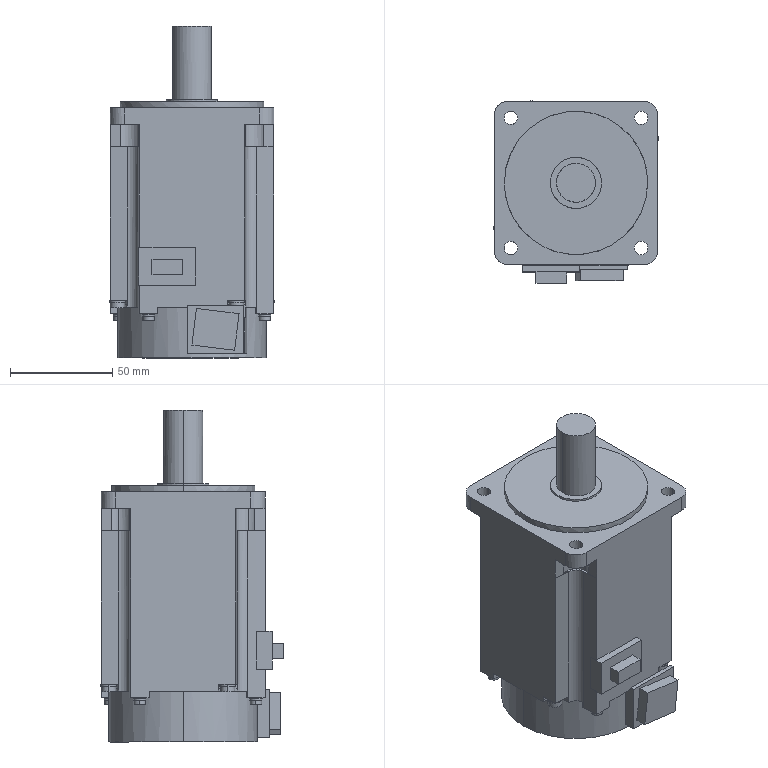Part | SolidWorks | features BaseBody 1 | 1 solid | 200 faces | box 80.44 x 89.02 x 162.2 mm | volume 690477 mm3 | plane 105 | cylinder 95 | commonest cylinder face diameters 920 x17 5.5 x8 5.9 x8 6 x8 6.6 x8 7 x8